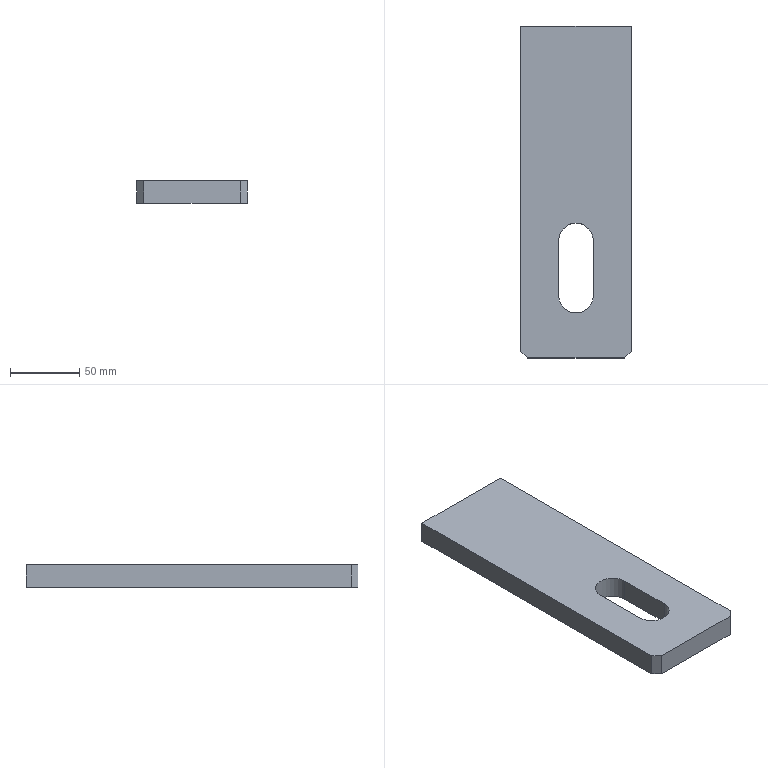Part | STEP file | 012-6-07-017 | 1 solid | 12 faces | box 80 x 240 x 16 mm | volume 282946 mm3 | plane 10 | cylinder 2 | commonest cylinder face diameters 25 x2
STEP:
#1=CARTESIAN_POINT('',(0.,0.,0.));
#2=DIRECTION('',(0.,0.,1.));
#3=DIRECTION('',(1.,0.,0.));
#4=AXIS2_PLACEMENT_3D('',#1,#2,#3);
#5=CARTESIAN_POINT('',(40.,-115.,16.));
#6=VERTEX_POINT('',#5);
#7=CARTESIAN_POINT('',(40.,120.,16.));
#8=VERTEX_POINT('',#7);
#9=CARTESIAN_POINT('',(40.,120.,16.));
#10=DIRECTION('',(0.,1.,0.));
#11=VECTOR('',#10,1.);
#12=LINE('',#9,#11);
#13=CARTESIAN_POINT('',(40.,120.,16.));
#14=DIRECTION('',(-1.,0.,0.));
#15=DIRECTION('',(0.,-1.,0.));
#16=AXIS2_PLACEMENT_3D('',#13,#14,#15);
#17=PLANE('',#16);
#18=CARTESIAN_POINT('',(0.,0.));
#19=DIRECTION('',(-1.,0.));
#20=VECTOR('',#19,1.);
#21=LINE('',#18,#20);
#22=(GEOMETRIC_REPRESENTATION_CONTEXT(2)PARAMETRIC_REPRESENTATION_CONTEXT()REPRESENTATION_CONTEXT('',''));
#23=DEFINITIONAL_REPRESENTATION('',(#21),#22);
#24=PCURVE('',#17,#23);
#25=CARTESIAN_POINT('',(40.,-120.,16.));
#26=DIRECTION('',(0.,0.,1.));
#27=DIRECTION('',(1.,0.,0.));
#28=AXIS2_PLACEMENT_3D('',#25,#26,#27);
#29=PLANE('',#28);
#30=CARTESIAN_POINT('',(0.,240.));
#31=DIRECTION('',(0.,1.));
#32=VECTOR('',#31,1.);
#33=LINE('',#30,#32);
#34=(GEOMETRIC_REPRESENTATION_CONTEXT(2)PARAMETRIC_REPRESENTATION_CONTEXT()REPRESENTATION_CONTEXT('',''));
#35=DEFINITIONAL_REPRESENTATION('',(#33),#34);
#36=PCURVE('',#29,#35);
#37=SURFACE_CURVE('',#12,(#24,#36),.PCURVE_S1.);
#38=EDGE_CURVE('',#6,#8,#37,.T.);
#39=ORIENTED_EDGE('',*,*,#38,.F.);
#40=CARTESIAN_POINT('',(40.,-115.,0.));
#41=VERTEX_POINT('',#40);
#42=CARTESIAN_POINT('',(40.,-115.,16.));
#43=DIRECTION('',(0.,0.,-1.));
#44=VECTOR('',#43,1.);
#45=LINE('',#42,#44);
#46=CARTESIAN_POINT('',(235.,0.));
#47=DIRECTION('',(0.,-1.));
#48=VECTOR('',#47,1.);
#49=LINE('',#46,#48);
#50=(GEOMETRIC_REPRESENTATION_CONTEXT(2)PARAMETRIC_REPRESENTATION_CONTEXT()REPRESENTATION_CONTEXT('',''));
#51=DEFINITIONAL_REPRESENTATION('',(#49),#50);
#52=PCURVE('',#17,#51);
#53=CARTESIAN_POINT('',(40.,-115.,16.));
#54=DIRECTION('',(-0.7071,0.7071,0.));
#55=DIRECTION('',(-0.7071,-0.7071,0.));
#56=AXIS2_PLACEMENT_3D('',#53,#54,#55);
#57=PLANE('',#56);
#58=CARTESIAN_POINT('',(0.,0.));
#59=DIRECTION('',(0.,-1.));
#60=VECTOR('',#59,1.);
#61=LINE('',#58,#60);
#62=(GEOMETRIC_REPRESENTATION_CONTEXT(2)PARAMETRIC_REPRESENTATION_CONTEXT()REPRESENTATION_CONTEXT('',''));
#63=DEFINITIONAL_REPRESENTATION('',(#61),#62);
#64=PCURVE('',#57,#63);
#65=SURFACE_CURVE('',#45,(#52,#64),.PCURVE_S1.);
#66=EDGE_CURVE('',#6,#41,#65,.T.);
#67=ORIENTED_EDGE('',*,*,#66,.T.);
#68=CARTESIAN_POINT('',(40.,120.,0.));
#69=VERTEX_POINT('',#68);
#70=CARTESIAN_POINT('',(40.,120.,0.));
#71=DIRECTION('',(0.,1.,0.));
#72=VECTOR('',#71,1.);
#73=LINE('',#70,#72);
#74=CARTESIAN_POINT('',(0.,-16.));
#75=DIRECTION('',(-1.,0.));
#76=VECTOR('',#75,1.);
#77=LINE('',#74,#76);
#78=(GEOMETRIC_REPRESENTATION_CONTEXT(2)PARAMETRIC_REPRESENTATION_CONTEXT()REPRESENTATION_CONTEXT('',''));
#79=DEFINITIONAL_REPRESENTATION('',(#77),#78);
#80=PCURVE('',#17,#79);
#81=CARTESIAN_POINT('',(40.,-120.,0.));
#82=DIRECTION('',(0.,0.,1.));
#83=DIRECTION('',(1.,0.,0.));
#84=AXIS2_PLACEMENT_3D('',#81,#82,#83);
#85=PLANE('',#84);
#86=CARTESIAN_POINT('',(0.,240.));
#87=DIRECTION('',(0.,1.));
#88=VECTOR('',#87,1.);
#89=LINE('',#86,#88);
#90=(GEOMETRIC_REPRESENTATION_CONTEXT(2)PARAMETRIC_REPRESENTATION_CONTEXT()REPRESENTATION_CONTEXT('',''));
#91=DEFINITIONAL_REPRESENTATION('',(#89),#90);
#92=PCURVE('',#85,#91);
#93=SURFACE_CURVE('',#73,(#80,#92),.PCURVE_S1.);
#94=EDGE_CURVE('',#41,#69,#93,.T.);
#95=ORIENTED_EDGE('',*,*,#94,.T.);
#96=CARTESIAN_POINT('',(40.,120.,16.));
#97=DIRECTION('',(0.,0.,-1.));
#98=VECTOR('',#97,1.);
#99=LINE('',#96,#98);
#100=CARTESIAN_POINT('',(0.,0.));
#101=DIRECTION('',(0.,-1.));
#102=VECTOR('',#101,1.);
#103=LINE('',#100,#102);
#104=(GEOMETRIC_REPRESENTATION_CONTEXT(2)PARAMETRIC_REPRESENTATION_CONTEXT()REPRESENTATION_CONTEXT('',''));
#105=DEFINITIONAL_REPRESENTATION('',(#103),#104);
#106=PCURVE('',#17,#105);
#107=CARTESIAN_POINT('',(-40.,120.,16.));
#108=DIRECTION('',(0.,-1.,0.));
#109=DIRECTION('',(0.,0.,-1.));
#110=AXIS2_PLACEMENT_3D('',#107,#108,#109);
#111=PLANE('',#110);
#112=CARTESIAN_POINT('',(0.,80.));
#113=DIRECTION('',(1.,0.));
#114=VECTOR('',#113,1.);
#115=LINE('',#112,#114);
#116=(GEOMETRIC_REPRESENTATION_CONTEXT(2)PARAMETRIC_REPRESENTATION_CONTEXT()REPRESENTATION_CONTEXT('',''));
#117=DEFINITIONAL_REPRESENTATION('',(#115),#116);
#118=PCURVE('',#111,#117);
#119=SURFACE_CURVE('',#99,(#106,#118),.PCURVE_S1.);
#120=EDGE_CURVE('',#8,#69,#119,.T.);
#121=ORIENTED_EDGE('',*,*,#120,.F.);
#122=EDGE_LOOP('',(#39,#67,#95,#121));
#123=FACE_BOUND('',#122,.T.);
#124=ADVANCED_FACE('',(#123),#17,.F.);
#125=CARTESIAN_POINT('',(-40.,120.,0.));
#126=VERTEX_POINT('',#125);
#127=CARTESIAN_POINT('',(-40.,120.,0.));
#128=DIRECTION('',(-1.,0.,0.));
#129=VECTOR('',#128,1.);
#130=LINE('',#127,#129);
#131=CARTESIAN_POINT('',(16.,0.));
#132=DIRECTION('',(0.,-1.));
#133=VECTOR('',#132,1.);
#134=LINE('',#131,#133);
#135=(GEOMETRIC_REPRESENTATION_CONTEXT(2)PARAMETRIC_REPRESENTATION_CONTEXT()REPRESENTATION_CONTEXT('',''));
#136=DEFINITIONAL_REPRESENTATION('',(#134),#135);
#137=PCURVE('',#111,#136);
#138=CARTESIAN_POINT('',(-80.,240.));
#139=DIRECTION('',(-1.,0.));
#140=VECTOR('',#139,1.);
#141=LINE('',#138,#140);
#142=(GEOMETRIC_REPRESENTATION_CONTEXT(2)PARAMETRIC_REPRESENTATION_CONTEXT()REPRESENTATION_CONTEXT('',''));
#143=DEFINITIONAL_REPRESENTATION('',(#141),#142);
#144=PCURVE('',#85,#143);
#145=SURFACE_CURVE('',#130,(#137,#144),.PCURVE_S1.);
#146=EDGE_CURVE('',#69,#126,#145,.T.);
#147=ORIENTED_EDGE('',*,*,#146,.T.);
#148=CARTESIAN_POINT('',(-40.,120.,16.));
#149=VERTEX_POINT('',#148);
#150=CARTESIAN_POINT('',(-40.,120.,16.));
#151=DIRECTION('',(0.,0.,-1.));
#152=VECTOR('',#151,1.);
#153=LINE('',#150,#152);
#154=CARTESIAN_POINT('',(0.,0.));
#155=DIRECTION('',(1.,0.));
#156=VECTOR('',#155,1.);
#157=LINE('',#154,#156);
#158=(GEOMETRIC_REPRESENTATION_CONTEXT(2)PARAMETRIC_REPRESENTATION_CONTEXT()REPRESENTATION_CONTEXT('',''));
#159=DEFINITIONAL_REPRESENTATION('',(#157),#158);
#160=PCURVE('',#111,#159);
#161=CARTESIAN_POINT('',(-40.,120.,16.));
#162=DIRECTION('',(1.,0.,0.));
#163=DIRECTION('',(0.,1.,0.));
#164=AXIS2_PLACEMENT_3D('',#161,#162,#163);
#165=PLANE('',#164);
#166=CARTESIAN_POINT('',(0.,0.));
#167=DIRECTION('',(0.,-1.));
#168=VECTOR('',#167,1.);
#169=LINE('',#166,#168);
#170=(GEOMETRIC_REPRESENTATION_CONTEXT(2)PARAMETRIC_REPRESENTATION_CONTEXT()REPRESENTATION_CONTEXT('',''));
#171=DEFINITIONAL_REPRESENTATION('',(#169),#170);
#172=PCURVE('',#165,#171);
#173=SURFACE_CURVE('',#153,(#160,#172),.PCURVE_S1.);
#174=EDGE_CURVE('',#149,#126,#173,.T.);
#175=ORIENTED_EDGE('',*,*,#174,.F.);
#176=CARTESIAN_POINT('',(-40.,120.,16.));
#177=DIRECTION('',(-1.,0.,0.));
#178=VECTOR('',#177,1.);
#179=LINE('',#176,#178);
#180=CARTESIAN_POINT('',(0.,0.));
#181=DIRECTION('',(0.,-1.));
#182=VECTOR('',#181,1.);
#183=LINE('',#180,#182);
#184=(GEOMETRIC_REPRESENTATION_CONTEXT(2)PARAMETRIC_REPRESENTATION_CONTEXT()REPRESENTATION_CONTEXT('',''));
#185=DEFINITIONAL_REPRESENTATION('',(#183),#184);
#186=PCURVE('',#111,#185);
#187=CARTESIAN_POINT('',(-80.,240.));
#188=DIRECTION('',(-1.,0.));
#189=VECTOR('',#188,1.);
#190=LINE('',#187,#189);
#191=(GEOMETRIC_REPRESENTATION_CONTEXT(2)PARAMETRIC_REPRESENTATION_CONTEXT()REPRESENTATION_CONTEXT('',''));
#192=DEFINITIONAL_REPRESENTATION('',(#190),#191);
#193=PCURVE('',#29,#192);
#194=SURFACE_CURVE('',#179,(#186,#193),.PCURVE_S1.);
#195=EDGE_CURVE('',#8,#149,#194,.T.);
#196=ORIENTED_EDGE('',*,*,#195,.F.);
#197=ORIENTED_EDGE('',*,*,#120,.T.);
#198=EDGE_LOOP('',(#147,#175,#196,#197));
#199=FACE_BOUND('',#198,.T.);
#200=ADVANCED_FACE('',(#199),#111,.F.);
#201=CARTESIAN_POINT('',(-40.,-115.,0.));
#202=VERTEX_POINT('',#201);
#203=CARTESIAN_POINT('',(-40.,120.,0.));
#204=DIRECTION('',(0.,-1.,0.));
#205=VECTOR('',#204,1.);
#206=LINE('',#203,#205);
#207=CARTESIAN_POINT('',(0.,-16.));
#208=DIRECTION('',(-1.,0.));
#209=VECTOR('',#208,1.);
#210=LINE('',#207,#209);
#211=(GEOMETRIC_REPRESENTATION_CONTEXT(2)PARAMETRIC_REPRESENTATION_CONTEXT()REPRESENTATION_CONTEXT('',''));
#212=DEFINITIONAL_REPRESENTATION('',(#210),#211);
#213=PCURVE('',#165,#212);
#214=CARTESIAN_POINT('',(-80.,240.));
#215=DIRECTION('',(0.,-1.));
#216=VECTOR('',#215,1.);
#217=LINE('',#214,#216);
#218=(GEOMETRIC_REPRESENTATION_CONTEXT(2)PARAMETRIC_REPRESENTATION_CONTEXT()REPRESENTATION_CONTEXT('',''));
#219=DEFINITIONAL_REPRESENTATION('',(#217),#218);
#220=PCURVE('',#85,#219);
#221=SURFACE_CURVE('',#206,(#213,#220),.PCURVE_S1.);
#222=EDGE_CURVE('',#126,#202,#221,.T.);
#223=ORIENTED_EDGE('',*,*,#222,.T.);
#224=CARTESIAN_POINT('',(-40.,-115.,16.));
#225=VERTEX_POINT('',#224);
#226=CARTESIAN_POINT('',(-40.,-115.,16.));
#227=DIRECTION('',(0.,0.,1.));
#228=VECTOR('',#227,1.);
#229=LINE('',#226,#228);
#230=CARTESIAN_POINT('',(-235.,0.));
#231=DIRECTION('',(0.,1.));
#232=VECTOR('',#231,1.);
#233=LINE('',#230,#232);
#234=(GEOMETRIC_REPRESENTATION_CONTEXT(2)PARAMETRIC_REPRESENTATION_CONTEXT()REPRESENTATION_CONTEXT('',''));
#235=DEFINITIONAL_REPRESENTATION('',(#233),#234);
#236=PCURVE('',#165,#235);
#237=CARTESIAN_POINT('',(-35.,-120.,16.));
#238=DIRECTION('',(0.7071,0.7071,0.));
#239=DIRECTION('',(-0.7071,0.7071,0.));
#240=AXIS2_PLACEMENT_3D('',#237,#238,#239);
#241=PLANE('',#240);
#242=CARTESIAN_POINT('',(7.071,0.));
#243=DIRECTION('',(0.,1.));
#244=VECTOR('',#243,1.);
#245=LINE('',#242,#244);
#246=(GEOMETRIC_REPRESENTATION_CONTEXT(2)PARAMETRIC_REPRESENTATION_CONTEXT()REPRESENTATION_CONTEXT('',''));
#247=DEFINITIONAL_REPRESENTATION('',(#245),#246);
#248=PCURVE('',#241,#247);
#249=SURFACE_CURVE('',#229,(#236,#248),.PCURVE_S1.);
#250=EDGE_CURVE('',#202,#225,#249,.T.);
#251=ORIENTED_EDGE('',*,*,#250,.T.);
#252=CARTESIAN_POINT('',(-40.,120.,16.));
#253=DIRECTION('',(0.,-1.,0.));
#254=VECTOR('',#253,1.);
#255=LINE('',#252,#254);
#256=CARTESIAN_POINT('',(0.,0.));
#257=DIRECTION('',(-1.,0.));
#258=VECTOR('',#257,1.);
#259=LINE('',#256,#258);
#260=(GEOMETRIC_REPRESENTATION_CONTEXT(2)PARAMETRIC_REPRESENTATION_CONTEXT()REPRESENTATION_CONTEXT('',''));
#261=DEFINITIONAL_REPRESENTATION('',(#259),#260);
#262=PCURVE('',#165,#261);
#263=CARTESIAN_POINT('',(-80.,240.));
#264=DIRECTION('',(0.,-1.));
#265=VECTOR('',#264,1.);
#266=LINE('',#263,#265);
#267=(GEOMETRIC_REPRESENTATION_CONTEXT(2)PARAMETRIC_REPRESENTATION_CONTEXT()REPRESENTATION_CONTEXT('',''));
#268=DEFINITIONAL_REPRESENTATION('',(#266),#267);
#269=PCURVE('',#29,#268);
#270=SURFACE_CURVE('',#255,(#262,#269),.PCURVE_S1.);
#271=EDGE_CURVE('',#149,#225,#270,.T.);
#272=ORIENTED_EDGE('',*,*,#271,.F.);
#273=ORIENTED_EDGE('',*,*,#174,.T.);
#274=EDGE_LOOP('',(#223,#251,#272,#273));
#275=FACE_BOUND('',#274,.T.);
#276=ADVANCED_FACE('',(#275),#165,.F.);
#277=CARTESIAN_POINT('',(-35.,-120.,16.));
#278=VERTEX_POINT('',#277);
#279=CARTESIAN_POINT('',(35.,-120.,16.));
#280=VERTEX_POINT('',#279);
#281=CARTESIAN_POINT('',(-40.,-120.,16.));
#282=DIRECTION('',(1.,0.,0.));
#283=VECTOR('',#282,1.);
#284=LINE('',#281,#283);
#285=CARTESIAN_POINT('',(-40.,-120.,16.));
#286=DIRECTION('',(0.,1.,0.));
#287=DIRECTION('',(0.,0.,1.));
#288=AXIS2_PLACEMENT_3D('',#285,#286,#287);
#289=PLANE('',#288);
#290=CARTESIAN_POINT('',(0.,0.));
#291=DIRECTION('',(0.,1.));
#292=VECTOR('',#291,1.);
#293=LINE('',#290,#292);
#294=(GEOMETRIC_REPRESENTATION_CONTEXT(2)PARAMETRIC_REPRESENTATION_CONTEXT()REPRESENTATION_CONTEXT('',''));
#295=DEFINITIONAL_REPRESENTATION('',(#293),#294);
#296=PCURVE('',#289,#295);
#297=CARTESIAN_POINT('',(-80.,0.));
#298=DIRECTION('',(1.,0.));
#299=VECTOR('',#298,1.);
#300=LINE('',#297,#299);
#301=(GEOMETRIC_REPRESENTATION_CONTEXT(2)PARAMETRIC_REPRESENTATION_CONTEXT()REPRESENTATION_CONTEXT('',''));
#302=DEFINITIONAL_REPRESENTATION('',(#300),#301);
#303=PCURVE('',#29,#302);
#304=SURFACE_CURVE('',#284,(#296,#303),.PCURVE_S1.);
#305=EDGE_CURVE('',#278,#280,#304,.T.);
#306=ORIENTED_EDGE('',*,*,#305,.F.);
#307=CARTESIAN_POINT('',(-35.,-120.,0.));
#308=VERTEX_POINT('',#307);
#309=CARTESIAN_POINT('',(-35.,-120.,16.));
#310=DIRECTION('',(0.,0.,-1.));
#311=VECTOR('',#310,1.);
#312=LINE('',#309,#311);
#313=CARTESIAN_POINT('',(0.,5.));
#314=DIRECTION('',(-1.,0.));
#315=VECTOR('',#314,1.);
#316=LINE('',#313,#315);
#317=(GEOMETRIC_REPRESENTATION_CONTEXT(2)PARAMETRIC_REPRESENTATION_CONTEXT()REPRESENTATION_CONTEXT('',''));
#318=DEFINITIONAL_REPRESENTATION('',(#316),#317);
#319=PCURVE('',#289,#318);
#320=CARTESIAN_POINT('',(0.,0.));
#321=DIRECTION('',(0.,-1.));
#322=VECTOR('',#321,1.);
#323=LINE('',#320,#322);
#324=(GEOMETRIC_REPRESENTATION_CONTEXT(2)PARAMETRIC_REPRESENTATION_CONTEXT()REPRESENTATION_CONTEXT('',''));
#325=DEFINITIONAL_REPRESENTATION('',(#323),#324);
#326=PCURVE('',#241,#325);
#327=SURFACE_CURVE('',#312,(#319,#326),.PCURVE_S1.);
#328=EDGE_CURVE('',#278,#308,#327,.T.);
#329=ORIENTED_EDGE('',*,*,#328,.T.);
#330=CARTESIAN_POINT('',(35.,-120.,0.));
#331=VERTEX_POINT('',#330);
#332=CARTESIAN_POINT('',(-40.,-120.,0.));
#333=DIRECTION('',(1.,0.,0.));
#334=VECTOR('',#333,1.);
#335=LINE('',#332,#334);
#336=CARTESIAN_POINT('',(-16.,0.));
#337=DIRECTION('',(0.,1.));
#338=VECTOR('',#337,1.);
#339=LINE('',#336,#338);
#340=(GEOMETRIC_REPRESENTATION_CONTEXT(2)PARAMETRIC_REPRESENTATION_CONTEXT()REPRESENTATION_CONTEXT('',''));
#341=DEFINITIONAL_REPRESENTATION('',(#339),#340);
#342=PCURVE('',#289,#341);
#343=CARTESIAN_POINT('',(-80.,0.));
#344=DIRECTION('',(1.,0.));
#345=VECTOR('',#344,1.);
#346=LINE('',#343,#345);
#347=(GEOMETRIC_REPRESENTATION_CONTEXT(2)PARAMETRIC_REPRESENTATION_CONTEXT()REPRESENTATION_CONTEXT('',''));
#348=DEFINITIONAL_REPRESENTATION('',(#346),#347);
#349=PCURVE('',#85,#348);
#350=SURFACE_CURVE('',#335,(#342,#349),.PCURVE_S1.);
#351=EDGE_CURVE('',#308,#331,#350,.T.);
#352=ORIENTED_EDGE('',*,*,#351,.T.);
#353=CARTESIAN_POINT('',(35.,-120.,16.));
#354=DIRECTION('',(0.,0.,1.));
#355=VECTOR('',#354,1.);
#356=LINE('',#353,#355);
#357=CARTESIAN_POINT('',(0.,75.));
#358=DIRECTION('',(1.,0.));
#359=VECTOR('',#358,1.);
#360=LINE('',#357,#359);
#361=(GEOMETRIC_REPRESENTATION_CONTEXT(2)PARAMETRIC_REPRESENTATION_CONTEXT()REPRESENTATION_CONTEXT('',''));
#362=DEFINITIONAL_REPRESENTATION('',(#360),#361);
#363=PCURVE('',#289,#362);
#364=CARTESIAN_POINT('',(7.071,0.));
#365=DIRECTION('',(0.,1.));
#366=VECTOR('',#365,1.);
#367=LINE('',#364,#366);
#368=(GEOMETRIC_REPRESENTATION_CONTEXT(2)PARAMETRIC_REPRESENTATION_CONTEXT()REPRESENTATION_CONTEXT('',''));
#369=DEFINITIONAL_REPRESENTATION('',(#367),#368);
#370=PCURVE('',#57,#369);
#371=SURFACE_CURVE('',#356,(#363,#370),.PCURVE_S1.);
#372=EDGE_CURVE('',#331,#280,#371,.T.);
#373=ORIENTED_EDGE('',*,*,#372,.T.);
#374=EDGE_LOOP('',(#306,#329,#352,#373));
#375=FACE_BOUND('',#374,.T.);
#376=ADVANCED_FACE('',(#375),#289,.F.);
#377=CARTESIAN_POINT('',(12.5,-35.,16.));
#378=VERTEX_POINT('',#377);
#379=CARTESIAN_POINT('',(-12.5,-35.,16.));
#380=VERTEX_POINT('',#379);
#381=CARTESIAN_POINT('',(0.,-35.,16.));
#382=DIRECTION('',(0.,0.,1.));
#383=DIRECTION('',(1.,0.,0.));
#384=AXIS2_PLACEMENT_3D('',#381,#382,#383);
#385=CIRCLE('',#384,12.5);
#386=CARTESIAN_POINT('',(-40.,85.));
#387=DIRECTION('',(1.,0.));
#388=AXIS2_PLACEMENT_2D('',#386,#387);
#389=CIRCLE('',#388,12.5);
#390=(GEOMETRIC_REPRESENTATION_CONTEXT(2)PARAMETRIC_REPRESENTATION_CONTEXT()REPRESENTATION_CONTEXT('',''));
#391=DEFINITIONAL_REPRESENTATION('',(#389),#390);
#392=PCURVE('',#29,#391);
#393=CARTESIAN_POINT('',(0.,-35.,18.));
#394=DIRECTION('',(0.,0.,-1.));
#395=DIRECTION('',(-1.,0.,0.));
#396=AXIS2_PLACEMENT_3D('',#393,#394,#395);
#397=CYLINDRICAL_SURFACE('',#396,12.5);
#398=CARTESIAN_POINT('',(3.142,2.));
#399=DIRECTION('',(-1.,0.));
#400=VECTOR('',#399,1.);
#401=LINE('',#398,#400);
#402=(GEOMETRIC_REPRESENTATION_CONTEXT(2)PARAMETRIC_REPRESENTATION_CONTEXT()REPRESENTATION_CONTEXT('',''));
#403=DEFINITIONAL_REPRESENTATION('',(#401),#402);
#404=PCURVE('',#397,#403);
#405=SURFACE_CURVE('',#385,(#392,#404),.PCURVE_S1.);
#406=EDGE_CURVE('',#378,#380,#405,.T.);
#407=ORIENTED_EDGE('',*,*,#406,.F.);
#408=CARTESIAN_POINT('',(12.5,-75.,16.));
#409=VERTEX_POINT('',#408);
#410=CARTESIAN_POINT('',(12.5,-120.,16.));
#411=DIRECTION('',(0.,1.,0.));
#412=VECTOR('',#411,1.);
#413=LINE('',#410,#412);
#414=CARTESIAN_POINT('',(-27.5,0.));
#415=DIRECTION('',(0.,1.));
#416=VECTOR('',#415,1.);
#417=LINE('',#414,#416);
#418=(GEOMETRIC_REPRESENTATION_CONTEXT(2)PARAMETRIC_REPRESENTATION_CONTEXT()REPRESENTATION_CONTEXT('',''));
#419=DEFINITIONAL_REPRESENTATION('',(#417),#418);
#420=PCURVE('',#29,#419);
#421=CARTESIAN_POINT('',(12.5,-35.,18.));
#422=DIRECTION('',(1.,0.,0.));
#423=DIRECTION('',(0.,1.,0.));
#424=AXIS2_PLACEMENT_3D('',#421,#422,#423);
#425=PLANE('',#424);
#426=CARTESIAN_POINT('',(-85.,-2.));
#427=DIRECTION('',(1.,0.));
#428=VECTOR('',#427,1.);
#429=LINE('',#426,#428);
#430=(GEOMETRIC_REPRESENTATION_CONTEXT(2)PARAMETRIC_REPRESENTATION_CONTEXT()REPRESENTATION_CONTEXT('',''));
#431=DEFINITIONAL_REPRESENTATION('',(#429),#430);
#432=PCURVE('',#425,#431);
#433=SURFACE_CURVE('',#413,(#420,#432),.PCURVE_S1.);
#434=EDGE_CURVE('',#409,#378,#433,.T.);
#435=ORIENTED_EDGE('',*,*,#434,.F.);
#436=CARTESIAN_POINT('',(-12.5,-75.,16.));
#437=VERTEX_POINT('',#436);
#438=CARTESIAN_POINT('',(0.,-75.,16.));
#439=DIRECTION('',(0.,0.,1.));
#440=DIRECTION('',(1.,0.,0.));
#441=AXIS2_PLACEMENT_3D('',#438,#439,#440);
#442=CIRCLE('',#441,12.5);
#443=CARTESIAN_POINT('',(-40.,45.));
#444=DIRECTION('',(1.,0.));
#445=AXIS2_PLACEMENT_2D('',#443,#444);
#446=CIRCLE('',#445,12.5);
#447=(GEOMETRIC_REPRESENTATION_CONTEXT(2)PARAMETRIC_REPRESENTATION_CONTEXT()REPRESENTATION_CONTEXT('',''));
#448=DEFINITIONAL_REPRESENTATION('',(#446),#447);
#449=PCURVE('',#29,#448);
#450=CARTESIAN_POINT('',(0.,-75.,18.));
#451=DIRECTION('',(0.,0.,-1.));
#452=DIRECTION('',(-1.,0.,0.));
#453=AXIS2_PLACEMENT_3D('',#450,#451,#452);
#454=CYLINDRICAL_SURFACE('',#453,12.5);
#455=CARTESIAN_POINT('',(9.425,2.));
#456=DIRECTION('',(-1.,0.));
#457=VECTOR('',#456,1.);
#458=LINE('',#455,#457);
#459=(GEOMETRIC_REPRESENTATION_CONTEXT(2)PARAMETRIC_REPRESENTATION_CONTEXT()REPRESENTATION_CONTEXT('',''));
#460=DEFINITIONAL_REPRESENTATION('',(#458),#459);
#461=PCURVE('',#454,#460);
#462=SURFACE_CURVE('',#442,(#449,#461),.PCURVE_S1.);
#463=EDGE_CURVE('',#437,#409,#462,.T.);
#464=ORIENTED_EDGE('',*,*,#463,.F.);
#465=CARTESIAN_POINT('',(-12.5,-120.,16.));
#466=DIRECTION('',(0.,-1.,0.));
#467=VECTOR('',#466,1.);
#468=LINE('',#465,#467);
#469=CARTESIAN_POINT('',(-52.5,0.));
#470=DIRECTION('',(0.,-1.));
#471=VECTOR('',#470,1.);
#472=LINE('',#469,#471);
#473=(GEOMETRIC_REPRESENTATION_CONTEXT(2)PARAMETRIC_REPRESENTATION_CONTEXT()REPRESENTATION_CONTEXT('',''));
#474=DEFINITIONAL_REPRESENTATION('',(#472),#473);
#475=PCURVE('',#29,#474);
#476=CARTESIAN_POINT('',(-12.5,-35.,18.));
#477=DIRECTION('',(-1.,0.,0.));
#478=DIRECTION('',(0.,-1.,0.));
#479=AXIS2_PLACEMENT_3D('',#476,#477,#478);
#480=PLANE('',#479);
#481=CARTESIAN_POINT('',(85.,-2.));
#482=DIRECTION('',(1.,0.));
#483=VECTOR('',#482,1.);
#484=LINE('',#481,#483);
#485=(GEOMETRIC_REPRESENTATION_CONTEXT(2)PARAMETRIC_REPRESENTATION_CONTEXT()REPRESENTATION_CONTEXT('',''));
#486=DEFINITIONAL_REPRESENTATION('',(#484),#485);
#487=PCURVE('',#480,#486);
#488=SURFACE_CURVE('',#468,(#475,#487),.PCURVE_S1.);
#489=EDGE_CURVE('',#380,#437,#488,.T.);
#490=ORIENTED_EDGE('',*,*,#489,.F.);
#491=EDGE_LOOP('',(#407,#435,#464,#490));
#492=FACE_BOUND('',#491,.T.);
#493=ORIENTED_EDGE('',*,*,#271,.T.);
#494=CARTESIAN_POINT('',(2.5,-157.5,16.));
#495=DIRECTION('',(0.7071,-0.7071,0.));
#496=VECTOR('',#495,1.);
#497=LINE('',#494,#496);
#498=CARTESIAN_POINT('',(-37.5,-37.5));
#499=DIRECTION('',(0.7071,-0.7071));
#500=VECTOR('',#499,1.);
#501=LINE('',#498,#500);
#502=(GEOMETRIC_REPRESENTATION_CONTEXT(2)PARAMETRIC_REPRESENTATION_CONTEXT()REPRESENTATION_CONTEXT('',''));
#503=DEFINITIONAL_REPRESENTATION('',(#501),#502);
#504=PCURVE('',#29,#503);
#505=CARTESIAN_POINT('',(-53.033,0.));
#506=DIRECTION('',(-1.,0.));
#507=VECTOR('',#506,1.);
#508=LINE('',#505,#507);
#509=(GEOMETRIC_REPRESENTATION_CONTEXT(2)PARAMETRIC_REPRESENTATION_CONTEXT()REPRESENTATION_CONTEXT('',''));
#510=DEFINITIONAL_REPRESENTATION('',(#508),#509);
#511=PCURVE('',#241,#510);
#512=SURFACE_CURVE('',#497,(#504,#511),.PCURVE_S1.);
#513=EDGE_CURVE('',#225,#278,#512,.T.);
#514=ORIENTED_EDGE('',*,*,#513,.T.);
#515=ORIENTED_EDGE('',*,*,#305,.T.);
#516=CARTESIAN_POINT('',(37.5,-117.5,16.));
#517=DIRECTION('',(0.7071,0.7071,0.));
#518=VECTOR('',#517,1.);
#519=LINE('',#516,#518);
#520=CARTESIAN_POINT('',(-2.5,2.5));
#521=DIRECTION('',(0.7071,0.7071));
#522=VECTOR('',#521,1.);
#523=LINE('',#520,#522);
#524=(GEOMETRIC_REPRESENTATION_CONTEXT(2)PARAMETRIC_REPRESENTATION_CONTEXT()REPRESENTATION_CONTEXT('',''));
#525=DEFINITIONAL_REPRESENTATION('',(#523),#524);
#526=PCURVE('',#29,#525);
#527=CARTESIAN_POINT('',(3.536,0.));
#528=DIRECTION('',(-1.,0.));
#529=VECTOR('',#528,1.);
#530=LINE('',#527,#529);
#531=(GEOMETRIC_REPRESENTATION_CONTEXT(2)PARAMETRIC_REPRESENTATION_CONTEXT()REPRESENTATION_CONTEXT('',''));
#532=DEFINITIONAL_REPRESENTATION('',(#530),#531);
#533=PCURVE('',#57,#532);
#534=SURFACE_CURVE('',#519,(#526,#533),.PCURVE_S1.);
#535=EDGE_CURVE('',#280,#6,#534,.T.);
#536=ORIENTED_EDGE('',*,*,#535,.T.);
#537=ORIENTED_EDGE('',*,*,#38,.T.);
#538=ORIENTED_EDGE('',*,*,#195,.T.);
#539=EDGE_LOOP('',(#493,#514,#515,#536,#537,#538));
#540=FACE_BOUND('',#539,.T.);
#541=ADVANCED_FACE('',(#492,#540),#29,.T.);
#542=CARTESIAN_POINT('',(12.5,-35.,0.));
#543=VERTEX_POINT('',#542);
#544=CARTESIAN_POINT('',(12.5,-75.,0.));
#545=VERTEX_POINT('',#544);
#546=CARTESIAN_POINT('',(12.5,-35.,0.));
#547=DIRECTION('',(0.,-1.,0.));
#548=VECTOR('',#547,1.);
#549=LINE('',#546,#548);
#550=CARTESIAN_POINT('',(-27.5,85.));
#551=DIRECTION('',(0.,-1.));
#552=VECTOR('',#551,1.);
#553=LINE('',#550,#552);
#554=(GEOMETRIC_REPRESENTATION_CONTEXT(2)PARAMETRIC_REPRESENTATION_CONTEXT()REPRESENTATION_CONTEXT('',''));
#555=DEFINITIONAL_REPRESENTATION('',(#553),#554);
#556=PCURVE('',#85,#555);
#557=CARTESIAN_POINT('',(0.,-18.));
#558=DIRECTION('',(-1.,0.));
#559=VECTOR('',#558,1.);
#560=LINE('',#557,#559);
#561=(GEOMETRIC_REPRESENTATION_CONTEXT(2)PARAMETRIC_REPRESENTATION_CONTEXT()REPRESENTATION_CONTEXT('',''));
#562=DEFINITIONAL_REPRESENTATION('',(#560),#561);
#563=PCURVE('',#425,#562);
#564=SURFACE_CURVE('',#549,(#556,#563),.PCURVE_S1.);
#565=EDGE_CURVE('',#543,#545,#564,.T.);
#566=ORIENTED_EDGE('',*,*,#565,.F.);
#567=CARTESIAN_POINT('',(-12.5,-35.,0.));
#568=VERTEX_POINT('',#567);
#569=CARTESIAN_POINT('',(0.,-35.,0.));
#570=DIRECTION('',(0.,0.,-1.));
#571=DIRECTION('',(-1.,0.,0.));
#572=AXIS2_PLACEMENT_3D('',#569,#570,#571);
#573=CIRCLE('',#572,12.5);
#574=CARTESIAN_POINT('',(-52.5,85.));
#575=CARTESIAN_POINT('',(-52.5,106.651));
#576=CARTESIAN_POINT('',(-33.75,95.825));
#577=CARTESIAN_POINT('',(-15.,85.));
#578=CARTESIAN_POINT('',(-33.75,74.175));
#579=CARTESIAN_POINT('',(-52.5,63.349));
#580=CARTESIAN_POINT('',(-52.5,85.));
#581=(BOUNDED_CURVE()B_SPLINE_CURVE(2,(#574,#575,#576,#577,#578,#579,#580),.UNSPECIFIED.,.T.,.F.)B_SPLINE_CURVE_WITH_KNOTS((1,2,2,2,2,1),(-2.094,0.,2.094,4.189,6.283,8.378),.UNSPECIFIED.)CURVE()GEOMETRIC_REPRESENTATION_ITEM()RATIONAL_B_SPLINE_CURVE((1.,0.5,1.,0.5,1.,0.5,1.))REPRESENTATION_ITEM(''));
#582=(GEOMETRIC_REPRESENTATION_CONTEXT(2)PARAMETRIC_REPRESENTATION_CONTEXT()REPRESENTATION_CONTEXT('',''));
#583=DEFINITIONAL_REPRESENTATION('',(#581),#582);
#584=PCURVE('',#85,#583);
#585=CARTESIAN_POINT('',(0.,18.));
#586=DIRECTION('',(1.,0.));
#587=VECTOR('',#586,1.);
#588=LINE('',#585,#587);
#589=(GEOMETRIC_REPRESENTATION_CONTEXT(2)PARAMETRIC_REPRESENTATION_CONTEXT()REPRESENTATION_CONTEXT('',''));
#590=DEFINITIONAL_REPRESENTATION('',(#588),#589);
#591=PCURVE('',#397,#590);
#592=SURFACE_CURVE('',#573,(#584,#591),.PCURVE_S1.);
#593=EDGE_CURVE('',#568,#543,#592,.T.);
#594=ORIENTED_EDGE('',*,*,#593,.F.);
#595=CARTESIAN_POINT('',(-12.5,-75.,0.));
#596=VERTEX_POINT('',#595);
#597=CARTESIAN_POINT('',(-12.5,-35.,0.));
#598=DIRECTION('',(0.,1.,0.));
#599=VECTOR('',#598,1.);
#600=LINE('',#597,#599);
#601=CARTESIAN_POINT('',(-52.5,85.));
#602=DIRECTION('',(0.,1.));
#603=VECTOR('',#602,1.);
#604=LINE('',#601,#603);
#605=(GEOMETRIC_REPRESENTATION_CONTEXT(2)PARAMETRIC_REPRESENTATION_CONTEXT()REPRESENTATION_CONTEXT('',''));
#606=DEFINITIONAL_REPRESENTATION('',(#604),#605);
#607=PCURVE('',#85,#606);
#608=CARTESIAN_POINT('',(0.,-18.));
#609=DIRECTION('',(-1.,0.));
#610=VECTOR('',#609,1.);
#611=LINE('',#608,#610);
#612=(GEOMETRIC_REPRESENTATION_CONTEXT(2)PARAMETRIC_REPRESENTATION_CONTEXT()REPRESENTATION_CONTEXT('',''));
#613=DEFINITIONAL_REPRESENTATION('',(#611),#612);
#614=PCURVE('',#480,#613);
#615=SURFACE_CURVE('',#600,(#607,#614),.PCURVE_S1.);
#616=EDGE_CURVE('',#596,#568,#615,.T.);
#617=ORIENTED_EDGE('',*,*,#616,.F.);
#618=CARTESIAN_POINT('',(0.,-75.,0.));
#619=DIRECTION('',(0.,0.,-1.));
#620=DIRECTION('',(-1.,0.,0.));
#621=AXIS2_PLACEMENT_3D('',#618,#619,#620);
#622=CIRCLE('',#621,12.5);
#623=CARTESIAN_POINT('',(-52.5,45.));
#624=CARTESIAN_POINT('',(-52.5,66.651));
#625=CARTESIAN_POINT('',(-33.75,55.825));
#626=CARTESIAN_POINT('',(-15.,45.));
#627=CARTESIAN_POINT('',(-33.75,34.175));
#628=CARTESIAN_POINT('',(-52.5,23.349));
#629=CARTESIAN_POINT('',(-52.5,45.));
#630=(BOUNDED_CURVE()B_SPLINE_CURVE(2,(#623,#624,#625,#626,#627,#628,#629),.UNSPECIFIED.,.T.,.F.)B_SPLINE_CURVE_WITH_KNOTS((1,2,2,2,2,1),(-2.094,0.,2.094,4.189,6.283,8.378),.UNSPECIFIED.)CURVE()GEOMETRIC_REPRESENTATION_ITEM()RATIONAL_B_SPLINE_CURVE((1.,0.5,1.,0.5,1.,0.5,1.))REPRESENTATION_ITEM(''));
#631=(GEOMETRIC_REPRESENTATION_CONTEXT(2)PARAMETRIC_REPRESENTATION_CONTEXT()REPRESENTATION_CONTEXT('',''));
#632=DEFINITIONAL_REPRESENTATION('',(#630),#631);
#633=PCURVE('',#85,#632);
#634=CARTESIAN_POINT('',(0.,18.));
#635=DIRECTION('',(1.,0.));
#636=VECTOR('',#635,1.);
#637=LINE('',#634,#636);
#638=(GEOMETRIC_REPRESENTATION_CONTEXT(2)PARAMETRIC_REPRESENTATION_CONTEXT()REPRESENTATION_CONTEXT('',''));
#639=DEFINITIONAL_REPRESENTATION('',(#637),#638);
#640=PCURVE('',#454,#639);
#641=SURFACE_CURVE('',#622,(#633,#640),.PCURVE_S1.);
#642=EDGE_CURVE('',#545,#596,#641,.T.);
#643=ORIENTED_EDGE('',*,*,#642,.F.);
#644=EDGE_LOOP('',(#566,#594,#617,#643));
#645=FACE_BOUND('',#644,.T.);
#646=ORIENTED_EDGE('',*,*,#351,.F.);
#647=CARTESIAN_POINT('',(-35.,-120.,0.));
#648=DIRECTION('',(-0.7071,0.7071,0.));
#649=VECTOR('',#648,1.);
#650=LINE('',#647,#649);
#651=CARTESIAN_POINT('',(-75.,0.));
#652=DIRECTION('',(-0.7071,0.7071));
#653=VECTOR('',#652,1.);
#654=LINE('',#651,#653);
#655=(GEOMETRIC_REPRESENTATION_CONTEXT(2)PARAMETRIC_REPRESENTATION_CONTEXT()REPRESENTATION_CONTEXT('',''));
#656=DEFINITIONAL_REPRESENTATION('',(#654),#655);
#657=PCURVE('',#85,#656);
#658=CARTESIAN_POINT('',(0.,-16.));
#659=DIRECTION('',(1.,0.));
#660=VECTOR('',#659,1.);
#661=LINE('',#658,#660);
#662=(GEOMETRIC_REPRESENTATION_CONTEXT(2)PARAMETRIC_REPRESENTATION_CONTEXT()REPRESENTATION_CONTEXT('',''));
#663=DEFINITIONAL_REPRESENTATION('',(#661),#662);
#664=PCURVE('',#241,#663);
#665=SURFACE_CURVE('',#650,(#657,#664),.PCURVE_S1.);
#666=EDGE_CURVE('',#308,#202,#665,.T.);
#667=ORIENTED_EDGE('',*,*,#666,.T.);
#668=ORIENTED_EDGE('',*,*,#222,.F.);
#669=ORIENTED_EDGE('',*,*,#146,.F.);
#670=ORIENTED_EDGE('',*,*,#94,.F.);
#671=CARTESIAN_POINT('',(40.,-115.,0.));
#672=DIRECTION('',(-0.7071,-0.7071,0.));
#673=VECTOR('',#672,1.);
#674=LINE('',#671,#673);
#675=CARTESIAN_POINT('',(0.,5.));
#676=DIRECTION('',(-0.7071,-0.7071));
#677=VECTOR('',#676,1.);
#678=LINE('',#675,#677);
#679=(GEOMETRIC_REPRESENTATION_CONTEXT(2)PARAMETRIC_REPRESENTATION_CONTEXT()REPRESENTATION_CONTEXT('',''));
#680=DEFINITIONAL_REPRESENTATION('',(#678),#679);
#681=PCURVE('',#85,#680);
#682=CARTESIAN_POINT('',(0.,-16.));
#683=DIRECTION('',(1.,0.));
#684=VECTOR('',#683,1.);
#685=LINE('',#682,#684);
#686=(GEOMETRIC_REPRESENTATION_CONTEXT(2)PARAMETRIC_REPRESENTATION_CONTEXT()REPRESENTATION_CONTEXT('',''));
#687=DEFINITIONAL_REPRESENTATION('',(#685),#686);
#688=PCURVE('',#57,#687);
#689=SURFACE_CURVE('',#674,(#681,#688),.PCURVE_S1.);
#690=EDGE_CURVE('',#41,#331,#689,.T.);
#691=ORIENTED_EDGE('',*,*,#690,.T.);
#692=EDGE_LOOP('',(#646,#667,#668,#669,#670,#691));
#693=FACE_BOUND('',#692,.T.);
#694=ADVANCED_FACE('',(#645,#693),#85,.F.);
#695=CARTESIAN_POINT('',(12.5,-35.,18.));
#696=DIRECTION('',(0.,0.,-1.));
#697=VECTOR('',#696,1.);
#698=LINE('',#695,#697);
#699=CARTESIAN_POINT('',(3.142,0.));
#700=DIRECTION('',(0.,1.));
#701=VECTOR('',#700,1.);
#702=LINE('',#699,#701);
#703=(GEOMETRIC_REPRESENTATION_CONTEXT(2)PARAMETRIC_REPRESENTATION_CONTEXT()REPRESENTATION_CONTEXT('',''));
#704=DEFINITIONAL_REPRESENTATION('',(#702),#703);
#705=PCURVE('',#397,#704);
#706=CARTESIAN_POINT('',(0.,0.));
#707=DIRECTION('',(0.,-1.));
#708=VECTOR('',#707,1.);
#709=LINE('',#706,#708);
#710=(GEOMETRIC_REPRESENTATION_CONTEXT(2)PARAMETRIC_REPRESENTATION_CONTEXT()REPRESENTATION_CONTEXT('',''));
#711=DEFINITIONAL_REPRESENTATION('',(#709),#710);
#712=PCURVE('',#425,#711);
#713=SURFACE_CURVE('',#698,(#705,#712),.PCURVE_S1.);
#714=EDGE_CURVE('',#378,#543,#713,.T.);
#715=ORIENTED_EDGE('',*,*,#714,.T.);
#716=ORIENTED_EDGE('',*,*,#593,.F.);
#717=CARTESIAN_POINT('',(-12.5,-35.,18.));
#718=DIRECTION('',(0.,0.,-1.));
#719=VECTOR('',#718,1.);
#720=LINE('',#717,#719);
#721=CARTESIAN_POINT('',(0.,0.));
#722=DIRECTION('',(0.,1.));
#723=VECTOR('',#722,1.);
#724=LINE('',#721,#723);
#725=(GEOMETRIC_REPRESENTATION_CONTEXT(2)PARAMETRIC_REPRESENTATION_CONTEXT()REPRESENTATION_CONTEXT('',''));
#726=DEFINITIONAL_REPRESENTATION('',(#724),#725);
#727=PCURVE('',#397,#726);
#728=CARTESIAN_POINT('',(0.,0.));
#729=DIRECTION('',(0.,-1.));
#730=VECTOR('',#729,1.);
#731=LINE('',#728,#730);
#732=(GEOMETRIC_REPRESENTATION_CONTEXT(2)PARAMETRIC_REPRESENTATION_CONTEXT()REPRESENTATION_CONTEXT('',''));
#733=DEFINITIONAL_REPRESENTATION('',(#731),#732);
#734=PCURVE('',#480,#733);
#735=SURFACE_CURVE('',#720,(#727,#734),.PCURVE_S1.);
#736=EDGE_CURVE('',#380,#568,#735,.T.);
#737=ORIENTED_EDGE('',*,*,#736,.F.);
#738=ORIENTED_EDGE('',*,*,#406,.F.);
#739=EDGE_LOOP('',(#715,#716,#737,#738));
#740=FACE_BOUND('',#739,.F.);
#741=ADVANCED_FACE('',(#740),#397,.F.);
#742=ORIENTED_EDGE('',*,*,#489,.T.);
#743=CARTESIAN_POINT('',(-12.5,-75.,18.));
#744=DIRECTION('',(0.,0.,-1.));
#745=VECTOR('',#744,1.);
#746=LINE('',#743,#745);
#747=CARTESIAN_POINT('',(40.,0.));
#748=DIRECTION('',(0.,-1.));
#749=VECTOR('',#748,1.);
#750=LINE('',#747,#749);
#751=(GEOMETRIC_REPRESENTATION_CONTEXT(2)PARAMETRIC_REPRESENTATION_CONTEXT()REPRESENTATION_CONTEXT('',''));
#752=DEFINITIONAL_REPRESENTATION('',(#750),#751);
#753=PCURVE('',#480,#752);
#754=CARTESIAN_POINT('',(6.283,0.));
#755=DIRECTION('',(0.,1.));
#756=VECTOR('',#755,1.);
#757=LINE('',#754,#756);
#758=(GEOMETRIC_REPRESENTATION_CONTEXT(2)PARAMETRIC_REPRESENTATION_CONTEXT()REPRESENTATION_CONTEXT('',''));
#759=DEFINITIONAL_REPRESENTATION('',(#757),#758);
#760=PCURVE('',#454,#759);
#761=SURFACE_CURVE('',#746,(#753,#760),.PCURVE_S1.);
#762=EDGE_CURVE('',#437,#596,#761,.T.);
#763=ORIENTED_EDGE('',*,*,#762,.T.);
#764=ORIENTED_EDGE('',*,*,#616,.T.);
#765=ORIENTED_EDGE('',*,*,#736,.F.);
#766=EDGE_LOOP('',(#742,#763,#764,#765));
#767=FACE_BOUND('',#766,.T.);
#768=ADVANCED_FACE('',(#767),#480,.F.);
#769=ORIENTED_EDGE('',*,*,#762,.T.);
#770=ORIENTED_EDGE('',*,*,#642,.F.);
#771=CARTESIAN_POINT('',(12.5,-75.,18.));
#772=DIRECTION('',(0.,0.,-1.));
#773=VECTOR('',#772,1.);
#774=LINE('',#771,#773);
#775=CARTESIAN_POINT('',(3.142,0.));
#776=DIRECTION('',(0.,1.));
#777=VECTOR('',#776,1.);
#778=LINE('',#775,#777);
#779=(GEOMETRIC_REPRESENTATION_CONTEXT(2)PARAMETRIC_REPRESENTATION_CONTEXT()REPRESENTATION_CONTEXT('',''));
#780=DEFINITIONAL_REPRESENTATION('',(#778),#779);
#781=PCURVE('',#454,#780);
#782=CARTESIAN_POINT('',(-40.,0.));
#783=DIRECTION('',(0.,-1.));
#784=VECTOR('',#783,1.);
#785=LINE('',#782,#784);
#786=(GEOMETRIC_REPRESENTATION_CONTEXT(2)PARAMETRIC_REPRESENTATION_CONTEXT()REPRESENTATION_CONTEXT('',''));
#787=DEFINITIONAL_REPRESENTATION('',(#785),#786);
#788=PCURVE('',#425,#787);
#789=SURFACE_CURVE('',#774,(#781,#788),.PCURVE_S1.);
#790=EDGE_CURVE('',#409,#545,#789,.T.);
#791=ORIENTED_EDGE('',*,*,#790,.F.);
#792=ORIENTED_EDGE('',*,*,#463,.F.);
#793=EDGE_LOOP('',(#769,#770,#791,#792));
#794=FACE_BOUND('',#793,.F.);
#795=ADVANCED_FACE('',(#794),#454,.F.);
#796=ORIENTED_EDGE('',*,*,#434,.T.);
#797=ORIENTED_EDGE('',*,*,#714,.T.);
#798=ORIENTED_EDGE('',*,*,#565,.T.);
#799=ORIENTED_EDGE('',*,*,#790,.F.);
#800=EDGE_LOOP('',(#796,#797,#798,#799));
#801=FACE_BOUND('',#800,.T.);
#802=ADVANCED_FACE('',(#801),#425,.F.);
#803=ORIENTED_EDGE('',*,*,#513,.F.);
#804=ORIENTED_EDGE('',*,*,#250,.F.);
#805=ORIENTED_EDGE('',*,*,#666,.F.);
#806=ORIENTED_EDGE('',*,*,#328,.F.);
#807=EDGE_LOOP('',(#803,#804,#805,#806));
#808=FACE_BOUND('',#807,.T.);
#809=ADVANCED_FACE('',(#808),#241,.F.);
#810=ORIENTED_EDGE('',*,*,#535,.F.);
#811=ORIENTED_EDGE('',*,*,#372,.F.);
#812=ORIENTED_EDGE('',*,*,#690,.F.);
#813=ORIENTED_EDGE('',*,*,#66,.F.);
#814=EDGE_LOOP('',(#810,#811,#812,#813));
#815=FACE_BOUND('',#814,.T.);
#816=ADVANCED_FACE('',(#815),#57,.F.);
#817=CLOSED_SHELL('',(#124,#200,#276,#376,#541,#694,#741,#768,#795,#802,#809,#816));
#818=MANIFOLD_SOLID_BREP('',#817);
#819=(LENGTH_UNIT()NAMED_UNIT(*)SI_UNIT(.MILLI.,.METRE.));
#820=UNCERTAINTY_MEASURE_WITH_UNIT(LENGTH_MEASURE(0.0000001),#819,'','');
#821=(NAMED_UNIT(*)PLANE_ANGLE_UNIT()SI_UNIT($,.RADIAN.));
#822=(NAMED_UNIT(*)SI_UNIT($,.STERADIAN.)SOLID_ANGLE_UNIT());
#823=(GEOMETRIC_REPRESENTATION_CONTEXT(3)GLOBAL_UNCERTAINTY_ASSIGNED_CONTEXT((#820))GLOBAL_UNIT_ASSIGNED_CONTEXT((#819,#821,#822))REPRESENTATION_CONTEXT('',''));
#824=ADVANCED_BREP_SHAPE_REPRESENTATION('',(#4,#818),#823);